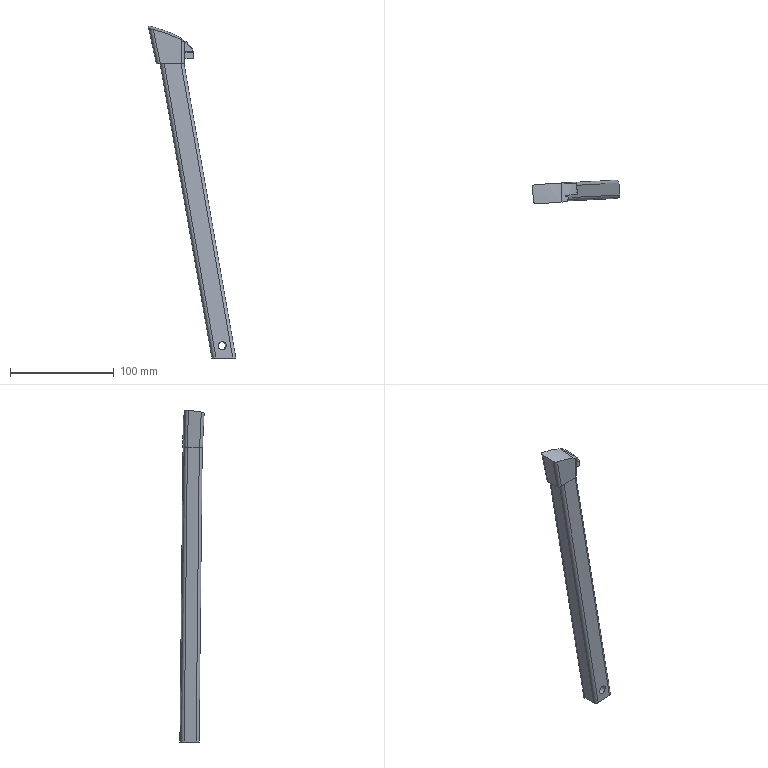Part | STEP file | 车灯-后视镜_id26_x_t | 1 solid | 48 faces | box 84.183 x 23.326 x 319.699 mm | volume 124323 mm3 | plane 34 | cylinder 8 | spline 6 | commonest cylinder face diameters 6 x7 8 x1